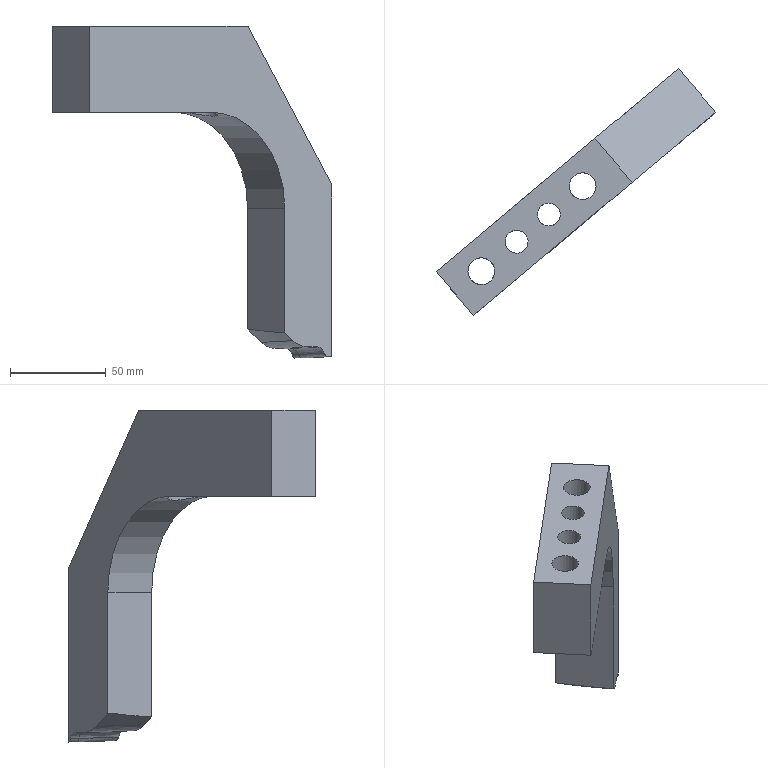Part | NX | features solid 2 | 1 solid | 26 faces | box 145.834 x 128.917 x 173.301 mm | volume 254338 mm3 | spline 10 | plane 9 | cylinder 7 | commonest cylinder face diameters 12 x2 14 x2 20 x2 100 x1